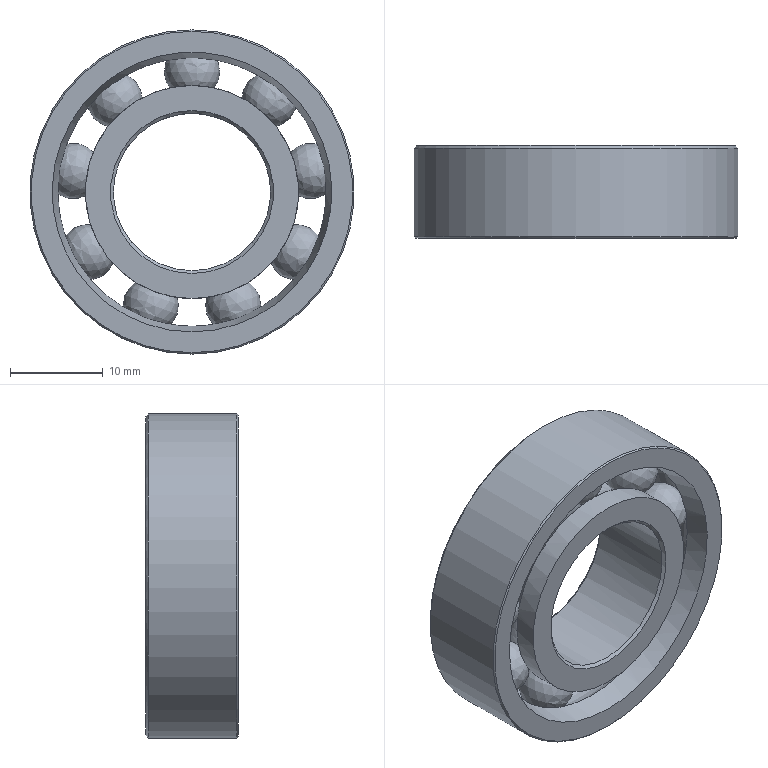Part | STEP file | 冲床-300配套压波_id266_x_t | 1 solid | 41 faces | box 35 x 10 x 35 mm | volume 4991 mm3 | torus 18 | sphere 9 | cylinder 5 | cone 5 | plane 4 | commonest cylinder face diameters 23 x2 17 x1 29 x1 35 x1